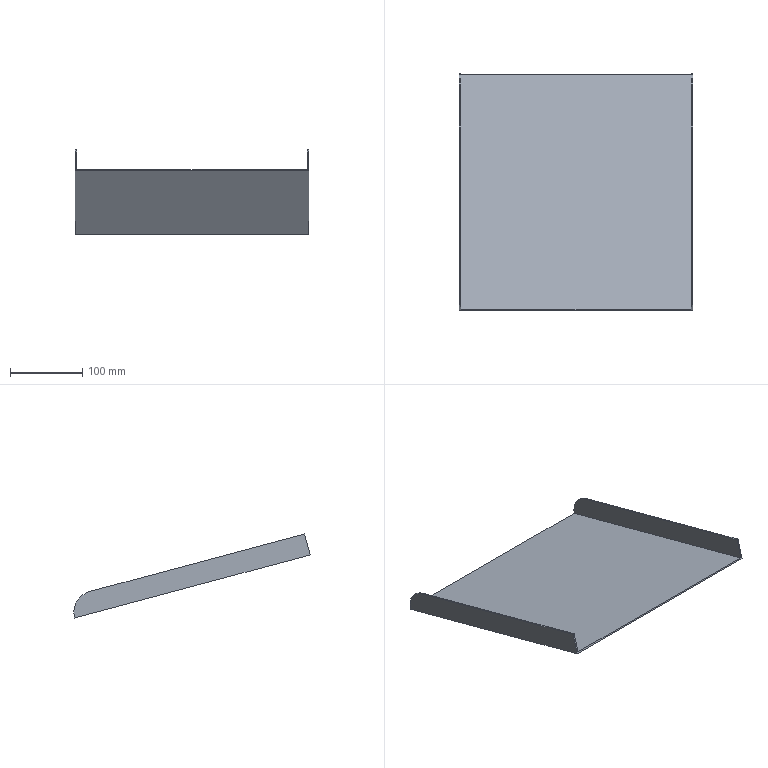Part | NX | features solid 2 | 1 solid | 12 faces | box 322.884 x 327.249 x 116.39 mm | volume 255152 mm3 | plane 9 | cylinder 2 | spline 1 | commonest cylinder face diameters 60 x2
STEP:
#1=CARTESIAN_POINT('',(-1268.,804.132,-484.555));
#2=VERTEX_POINT('',#1);
#3=CARTESIAN_POINT('',(-1268.,1130.294,-571.95));
#4=VERTEX_POINT('',#3);
#5=CARTESIAN_POINT('',(-1268.,966.151,-527.968));
#6=DIRECTION('',(0.,0.9659,-0.2588));
#7=VECTOR('',#6,1000.);
#8=LINE('',#5,#7);
#9=EDGE_CURVE('',#2,#4,#8,.T.);
#10=ORIENTED_EDGE('',*,*,#9,.F.);
#11=CARTESIAN_POINT('',(-949.116,804.132,-484.555));
#12=VERTEX_POINT('',#11);
#13=CARTESIAN_POINT('',(-1258.,804.132,-484.555));
#14=DIRECTION('',(1.,0.,0.));
#15=VECTOR('',#14,1000.);
#16=LINE('',#13,#15);
#17=EDGE_CURVE('',#2,#12,#16,.T.);
#18=ORIENTED_EDGE('',*,*,#17,.T.);
#19=CARTESIAN_POINT('',(-949.116,1130.294,-571.95));
#20=VERTEX_POINT('',#19);
#21=CARTESIAN_POINT('',(-949.116,966.151,-527.968));
#22=DIRECTION('',(0.,0.9659,-0.2588));
#23=VECTOR('',#22,1000.);
#24=LINE('',#21,#23);
#25=EDGE_CURVE('',#12,#20,#24,.T.);
#26=ORIENTED_EDGE('',*,*,#25,.T.);
#27=CARTESIAN_POINT('',(-947.116,1130.294,-571.95));
#28=VERTEX_POINT('',#27);
#29=CARTESIAN_POINT('',(-947.116,1130.294,-571.95));
#30=DIRECTION('',(1.,0.,0.));
#31=VECTOR('',#30,1000.);
#32=LINE('',#29,#31);
#33=EDGE_CURVE('',#28,#20,#32,.F.);
#34=ORIENTED_EDGE('',*,*,#33,.F.);
#35=CARTESIAN_POINT('',(-947.116,1130.359,-571.967));
#36=VERTEX_POINT('',#35);
#37=CARTESIAN_POINT('',(-947.116,966.151,-527.968));
#38=DIRECTION('',(0.,-0.9659,0.2588));
#39=VECTOR('',#38,1000.);
#40=LINE('',#37,#39);
#41=EDGE_CURVE('',#28,#36,#40,.F.);
#42=ORIENTED_EDGE('',*,*,#41,.T.);
#43=CARTESIAN_POINT('',(-1270.,1130.359,-571.967));
#44=VERTEX_POINT('',#43);
#45=CARTESIAN_POINT('',(-1302.833,1130.359,-571.967));
#46=CARTESIAN_POINT('',(-1258.,1130.359,-571.967));
#47=CARTESIAN_POINT('',(-959.116,1130.359,-571.967));
#48=CARTESIAN_POINT('',(-914.283,1130.359,-571.967));
#49=B_SPLINE_CURVE_WITH_KNOTS('',1,(#45,#46,#47,#48),.UNSPECIFIED.,.F.,.F.,(2,1,1,2),(-0.15,0.,1.,1.15),.PIECEWISE_BEZIER_KNOTS.);
#50=EDGE_CURVE('',#44,#36,#49,.T.);
#51=ORIENTED_EDGE('',*,*,#50,.F.);
#52=CARTESIAN_POINT('',(-1270.,1130.294,-571.95));
#53=VERTEX_POINT('',#52);
#54=CARTESIAN_POINT('',(-1270.,966.151,-527.968));
#55=DIRECTION('',(0.,0.9659,-0.2588));
#56=VECTOR('',#55,1000.);
#57=LINE('',#54,#56);
#58=EDGE_CURVE('',#53,#44,#57,.T.);
#59=ORIENTED_EDGE('',*,*,#58,.F.);
#60=CARTESIAN_POINT('',(-1270.,1130.294,-571.95));
#61=DIRECTION('',(-1.,0.,0.));
#62=VECTOR('',#61,1000.);
#63=LINE('',#60,#62);
#64=EDGE_CURVE('',#4,#53,#63,.T.);
#65=ORIENTED_EDGE('',*,*,#64,.F.);
#66=EDGE_LOOP('',(#10,#18,#26,#34,#42,#51,#59,#65));
#67=FACE_BOUND('',#66,.T.);
#68=CARTESIAN_POINT('',(-1258.,966.151,-527.968));
#69=DIRECTION('',(0.,0.2588,0.9659));
#70=DIRECTION('',(1.,0.,0.));
#71=AXIS2_PLACEMENT_3D('',#68,#69,#70);
#72=PLANE('',#71);
#73=ADVANCED_FACE('',(#67),#72,.T.);
#74=CARTESIAN_POINT('',(-947.116,803.615,-486.487));
#75=VERTEX_POINT('',#74);
#76=CARTESIAN_POINT('',(-947.116,811.379,-457.509));
#77=VERTEX_POINT('',#76);
#78=CARTESIAN_POINT('',(-947.116,804.132,-484.555));
#79=DIRECTION('',(0.,-0.2588,-0.9659));
#80=VECTOR('',#79,1000.);
#81=LINE('',#78,#80);
#82=EDGE_CURVE('',#75,#77,#81,.F.);
#83=ORIENTED_EDGE('',*,*,#82,.F.);
#84=CARTESIAN_POINT('',(-947.116,1129.841,-573.899));
#85=VERTEX_POINT('',#84);
#86=CARTESIAN_POINT('',(-947.116,965.634,-529.9));
#87=DIRECTION('',(0.,-0.9659,0.2588));
#88=VECTOR('',#87,1000.);
#89=LINE('',#86,#88);
#90=EDGE_CURVE('',#75,#85,#89,.F.);
#91=ORIENTED_EDGE('',*,*,#90,.T.);
#92=CARTESIAN_POINT('',(-947.116,1130.1,-572.933));
#93=DIRECTION('',(0.,0.2588,0.9659));
#94=VECTOR('',#93,1000.);
#95=LINE('',#92,#94);
#96=EDGE_CURVE('',#36,#85,#95,.F.);
#97=ORIENTED_EDGE('',*,*,#96,.F.);
#98=ORIENTED_EDGE('',*,*,#41,.F.);
#99=CARTESIAN_POINT('',(-947.116,1108.628,-537.157));
#100=VERTEX_POINT('',#99);
#101=CARTESIAN_POINT('',(-947.116,1100.863,-566.134));
#102=DIRECTION('',(1.,0.,0.));
#103=DIRECTION('',(0.,0.08716,-0.9962));
#104=AXIS2_PLACEMENT_3D('',#101,#102,#103);
#105=CIRCLE('',#104,30.);
#106=EDGE_CURVE('',#28,#100,#105,.T.);
#107=ORIENTED_EDGE('',*,*,#106,.T.);
#108=CARTESIAN_POINT('',(-947.116,944.421,-493.157));
#109=DIRECTION('',(0.,0.9659,-0.2588));
#110=VECTOR('',#109,1000.);
#111=LINE('',#108,#110);
#112=EDGE_CURVE('',#77,#100,#111,.T.);
#113=ORIENTED_EDGE('',*,*,#112,.F.);
#114=EDGE_LOOP('',(#83,#91,#97,#98,#107,#113));
#115=FACE_BOUND('',#114,.T.);
#116=CARTESIAN_POINT('',(-947.116,966.151,-527.968));
#117=DIRECTION('',(1.,0.,0.));
#118=DIRECTION('',(0.,0.9659,-0.2588));
#119=AXIS2_PLACEMENT_3D('',#116,#117,#118);
#120=PLANE('',#119);
#121=ADVANCED_FACE('',(#115),#120,.T.);
#122=CARTESIAN_POINT('',(-1270.,811.379,-457.509));
#123=VERTEX_POINT('',#122);
#124=CARTESIAN_POINT('',(-1270.,803.615,-486.487));
#125=VERTEX_POINT('',#124);
#126=CARTESIAN_POINT('',(-1270.,804.132,-484.555));
#127=DIRECTION('',(0.,-0.2588,-0.9659));
#128=VECTOR('',#127,1000.);
#129=LINE('',#126,#128);
#130=EDGE_CURVE('',#123,#125,#129,.T.);
#131=ORIENTED_EDGE('',*,*,#130,.F.);
#132=CARTESIAN_POINT('',(-1270.,1108.628,-537.157));
#133=VERTEX_POINT('',#132);
#134=CARTESIAN_POINT('',(-1270.,944.421,-493.157));
#135=DIRECTION('',(0.,0.9659,-0.2588));
#136=VECTOR('',#135,1000.);
#137=LINE('',#134,#136);
#138=EDGE_CURVE('',#123,#133,#137,.T.);
#139=ORIENTED_EDGE('',*,*,#138,.T.);
#140=CARTESIAN_POINT('',(-1270.,1100.863,-566.134));
#141=DIRECTION('',(1.,0.,0.));
#142=DIRECTION('',(0.,0.08716,-0.9962));
#143=AXIS2_PLACEMENT_3D('',#140,#141,#142);
#144=CIRCLE('',#143,30.);
#145=EDGE_CURVE('',#133,#53,#144,.F.);
#146=ORIENTED_EDGE('',*,*,#145,.T.);
#147=ORIENTED_EDGE('',*,*,#58,.T.);
#148=CARTESIAN_POINT('',(-1270.,1129.841,-573.899));
#149=VERTEX_POINT('',#148);
#150=CARTESIAN_POINT('',(-1270.,1130.359,-571.967));
#151=DIRECTION('',(0.,0.2588,0.9659));
#152=VECTOR('',#151,1000.);
#153=LINE('',#150,#152);
#154=EDGE_CURVE('',#44,#149,#153,.F.);
#155=ORIENTED_EDGE('',*,*,#154,.T.);
#156=CARTESIAN_POINT('',(-1270.,965.634,-529.9));
#157=DIRECTION('',(0.,0.9659,-0.2588));
#158=VECTOR('',#157,1000.);
#159=LINE('',#156,#158);
#160=EDGE_CURVE('',#125,#149,#159,.T.);
#161=ORIENTED_EDGE('',*,*,#160,.F.);
#162=EDGE_LOOP('',(#131,#139,#146,#147,#155,#161));
#163=FACE_BOUND('',#162,.T.);
#164=CARTESIAN_POINT('',(-1270.,966.151,-527.968));
#165=DIRECTION('',(1.,0.,0.));
#166=DIRECTION('',(0.,0.9659,-0.2588));
#167=AXIS2_PLACEMENT_3D('',#164,#165,#166);
#168=PLANE('',#167);
#169=ADVANCED_FACE('',(#163),#168,.F.);
#170=CARTESIAN_POINT('',(-1258.,803.615,-486.487));
#171=DIRECTION('',(1.,0.,0.));
#172=VECTOR('',#171,1000.);
#173=LINE('',#170,#172);
#174=EDGE_CURVE('',#125,#75,#173,.T.);
#175=ORIENTED_EDGE('',*,*,#174,.F.);
#176=ORIENTED_EDGE('',*,*,#160,.T.);
#177=CARTESIAN_POINT('',(-1302.833,1129.841,-573.899));
#178=CARTESIAN_POINT('',(-1258.,1129.841,-573.899));
#179=CARTESIAN_POINT('',(-959.116,1129.841,-573.899));
#180=CARTESIAN_POINT('',(-914.283,1129.841,-573.899));
#181=B_SPLINE_CURVE_WITH_KNOTS('',1,(#177,#178,#179,#180),.UNSPECIFIED.,.F.,.F.,(2,1,1,2),(-0.15,0.,1.,1.15),.PIECEWISE_BEZIER_KNOTS.);
#182=EDGE_CURVE('',#149,#85,#181,.T.);
#183=ORIENTED_EDGE('',*,*,#182,.T.);
#184=ORIENTED_EDGE('',*,*,#90,.F.);
#185=EDGE_LOOP('',(#175,#176,#183,#184));
#186=FACE_BOUND('',#185,.T.);
#187=CARTESIAN_POINT('',(-1258.,965.634,-529.9));
#188=DIRECTION('',(0.,0.2588,0.9659));
#189=DIRECTION('',(1.,0.,0.));
#190=AXIS2_PLACEMENT_3D('',#187,#188,#189);
#191=PLANE('',#190);
#192=ADVANCED_FACE('',(#186),#191,.F.);
#193=CARTESIAN_POINT('',(-949.116,811.379,-457.509));
#194=VERTEX_POINT('',#193);
#195=CARTESIAN_POINT('',(-947.116,811.379,-457.509));
#196=DIRECTION('',(-1.,0.,0.));
#197=VECTOR('',#196,1000.);
#198=LINE('',#195,#197);
#199=EDGE_CURVE('',#77,#194,#198,.T.);
#200=ORIENTED_EDGE('',*,*,#199,.F.);
#201=ORIENTED_EDGE('',*,*,#112,.T.);
#202=CARTESIAN_POINT('',(-949.116,1108.628,-537.157));
#203=VERTEX_POINT('',#202);
#204=CARTESIAN_POINT('',(-947.116,1108.628,-537.157));
#205=DIRECTION('',(1.,0.,0.));
#206=VECTOR('',#205,1000.);
#207=LINE('',#204,#206);
#208=EDGE_CURVE('',#100,#203,#207,.F.);
#209=ORIENTED_EDGE('',*,*,#208,.T.);
#210=CARTESIAN_POINT('',(-949.116,944.421,-493.157));
#211=DIRECTION('',(0.,0.9659,-0.2588));
#212=VECTOR('',#211,1000.);
#213=LINE('',#210,#212);
#214=EDGE_CURVE('',#194,#203,#213,.T.);
#215=ORIENTED_EDGE('',*,*,#214,.F.);
#216=EDGE_LOOP('',(#200,#201,#209,#215));
#217=FACE_BOUND('',#216,.T.);
#218=CARTESIAN_POINT('',(-947.116,944.421,-493.157));
#219=DIRECTION('',(0.,-0.2588,-0.9659));
#220=DIRECTION('',(0.,0.9659,-0.2588));
#221=AXIS2_PLACEMENT_3D('',#218,#219,#220);
#222=PLANE('',#221);
#223=ADVANCED_FACE('',(#217),#222,.F.);
#224=CARTESIAN_POINT('',(-949.116,803.615,-486.487));
#225=DIRECTION('',(0.,-0.2588,-0.9659));
#226=VECTOR('',#225,1000.);
#227=LINE('',#224,#226);
#228=EDGE_CURVE('',#194,#12,#227,.T.);
#229=ORIENTED_EDGE('',*,*,#228,.F.);
#230=ORIENTED_EDGE('',*,*,#214,.T.);
#231=CARTESIAN_POINT('',(-949.116,1100.863,-566.134));
#232=DIRECTION('',(1.,0.,0.));
#233=DIRECTION('',(0.,0.08716,-0.9962));
#234=AXIS2_PLACEMENT_3D('',#231,#232,#233);
#235=CIRCLE('',#234,30.);
#236=EDGE_CURVE('',#203,#20,#235,.F.);
#237=ORIENTED_EDGE('',*,*,#236,.T.);
#238=ORIENTED_EDGE('',*,*,#25,.F.);
#239=EDGE_LOOP('',(#229,#230,#237,#238));
#240=FACE_BOUND('',#239,.T.);
#241=CARTESIAN_POINT('',(-949.116,936.656,-522.135));
#242=DIRECTION('',(1.,0.,0.));
#243=DIRECTION('',(0.,0.08716,-0.9962));
#244=AXIS2_PLACEMENT_3D('',#241,#242,#243);
#245=PLANE('',#244);
#246=ADVANCED_FACE('',(#240),#245,.F.);
#247=ORIENTED_EDGE('',*,*,#138,.F.);
#248=CARTESIAN_POINT('',(-1268.,811.379,-457.509));
#249=VERTEX_POINT('',#248);
#250=CARTESIAN_POINT('',(-1270.,811.379,-457.509));
#251=DIRECTION('',(-1.,0.,0.));
#252=VECTOR('',#251,1000.);
#253=LINE('',#250,#252);
#254=EDGE_CURVE('',#123,#249,#253,.F.);
#255=ORIENTED_EDGE('',*,*,#254,.T.);
#256=CARTESIAN_POINT('',(-1268.,1108.628,-537.157));
#257=VERTEX_POINT('',#256);
#258=CARTESIAN_POINT('',(-1268.,944.421,-493.157));
#259=DIRECTION('',(0.,0.9659,-0.2588));
#260=VECTOR('',#259,1000.);
#261=LINE('',#258,#260);
#262=EDGE_CURVE('',#249,#257,#261,.T.);
#263=ORIENTED_EDGE('',*,*,#262,.T.);
#264=CARTESIAN_POINT('',(-1270.,1108.628,-537.157));
#265=DIRECTION('',(1.,0.,0.));
#266=VECTOR('',#265,1000.);
#267=LINE('',#264,#266);
#268=EDGE_CURVE('',#257,#133,#267,.F.);
#269=ORIENTED_EDGE('',*,*,#268,.T.);
#270=EDGE_LOOP('',(#247,#255,#263,#269));
#271=FACE_BOUND('',#270,.T.);
#272=CARTESIAN_POINT('',(-1270.,944.421,-493.157));
#273=DIRECTION('',(0.,-0.2588,-0.9659));
#274=DIRECTION('',(0.,0.9659,-0.2588));
#275=AXIS2_PLACEMENT_3D('',#272,#273,#274);
#276=PLANE('',#275);
#277=ADVANCED_FACE('',(#271),#276,.F.);
#278=ORIENTED_EDGE('',*,*,#262,.F.);
#279=CARTESIAN_POINT('',(-1268.,803.615,-486.487));
#280=DIRECTION('',(0.,-0.2588,-0.9659));
#281=VECTOR('',#280,1000.);
#282=LINE('',#279,#281);
#283=EDGE_CURVE('',#249,#2,#282,.T.);
#284=ORIENTED_EDGE('',*,*,#283,.T.);
#285=ORIENTED_EDGE('',*,*,#9,.T.);
#286=CARTESIAN_POINT('',(-1268.,1100.863,-566.134));
#287=DIRECTION('',(1.,0.,0.));
#288=DIRECTION('',(0.,0.08716,-0.9962));
#289=AXIS2_PLACEMENT_3D('',#286,#287,#288);
#290=CIRCLE('',#289,30.);
#291=EDGE_CURVE('',#4,#257,#290,.T.);
#292=ORIENTED_EDGE('',*,*,#291,.T.);
#293=EDGE_LOOP('',(#278,#284,#285,#292));
#294=FACE_BOUND('',#293,.T.);
#295=CARTESIAN_POINT('',(-1268.,936.656,-522.135));
#296=DIRECTION('',(1.,0.,0.));
#297=DIRECTION('',(0.,0.08716,-0.9962));
#298=AXIS2_PLACEMENT_3D('',#295,#296,#297);
#299=PLANE('',#298);
#300=ADVANCED_FACE('',(#294),#299,.T.);
#301=ORIENTED_EDGE('',*,*,#96,.T.);
#302=ORIENTED_EDGE('',*,*,#182,.F.);
#303=ORIENTED_EDGE('',*,*,#154,.F.);
#304=ORIENTED_EDGE('',*,*,#50,.T.);
#305=EDGE_LOOP('',(#301,#302,#303,#304));
#306=FACE_BOUND('',#305,.T.);
#307=CARTESIAN_POINT('',(-1270.,1129.841,-573.899));
#308=CARTESIAN_POINT('',(-1270.,1130.359,-571.967));
#309=CARTESIAN_POINT('',(-1258.,1129.841,-573.899));
#310=CARTESIAN_POINT('',(-1258.,1130.359,-571.967));
#311=CARTESIAN_POINT('',(-959.116,1129.841,-573.899));
#312=CARTESIAN_POINT('',(-959.116,1130.359,-571.967));
#313=CARTESIAN_POINT('',(-947.116,1129.841,-573.899));
#314=CARTESIAN_POINT('',(-947.116,1130.359,-571.967));
#315=B_SPLINE_SURFACE_WITH_KNOTS('',1,1,((#307,#308),(#309,#310),(#311,#312),(#313,#314)),.SURF_OF_LINEAR_EXTRUSION.,.F.,.F.,.F.,(2,1,1,2),(2,2),(-0.04015,0.,1.,1.04),(0.,1.),.PIECEWISE_BEZIER_KNOTS.);
#316=ADVANCED_FACE('',(#306),#315,.F.);
#317=ORIENTED_EDGE('',*,*,#106,.F.);
#318=ORIENTED_EDGE('',*,*,#33,.T.);
#319=ORIENTED_EDGE('',*,*,#236,.F.);
#320=ORIENTED_EDGE('',*,*,#208,.F.);
#321=EDGE_LOOP('',(#317,#318,#319,#320));
#322=FACE_BOUND('',#321,.T.);
#323=CARTESIAN_POINT('',(-947.116,1100.863,-566.134));
#324=DIRECTION('',(1.,0.,0.));
#325=DIRECTION('',(0.,0.08716,-0.9962));
#326=AXIS2_PLACEMENT_3D('',#323,#324,#325);
#327=CYLINDRICAL_SURFACE('',#326,30.);
#328=ADVANCED_FACE('',(#322),#327,.T.);
#329=ORIENTED_EDGE('',*,*,#291,.F.);
#330=ORIENTED_EDGE('',*,*,#64,.T.);
#331=ORIENTED_EDGE('',*,*,#145,.F.);
#332=ORIENTED_EDGE('',*,*,#268,.F.);
#333=EDGE_LOOP('',(#329,#330,#331,#332));
#334=FACE_BOUND('',#333,.T.);
#335=CARTESIAN_POINT('',(-1270.,1100.863,-566.134));
#336=DIRECTION('',(-1.,0.,0.));
#337=DIRECTION('',(0.,-0.08716,0.9962));
#338=AXIS2_PLACEMENT_3D('',#335,#336,#337);
#339=CYLINDRICAL_SURFACE('',#338,30.);
#340=ADVANCED_FACE('',(#334),#339,.T.);
#341=ORIENTED_EDGE('',*,*,#174,.T.);
#342=ORIENTED_EDGE('',*,*,#82,.T.);
#343=ORIENTED_EDGE('',*,*,#199,.T.);
#344=ORIENTED_EDGE('',*,*,#228,.T.);
#345=ORIENTED_EDGE('',*,*,#17,.F.);
#346=ORIENTED_EDGE('',*,*,#283,.F.);
#347=ORIENTED_EDGE('',*,*,#254,.F.);
#348=ORIENTED_EDGE('',*,*,#130,.T.);
#349=EDGE_LOOP('',(#341,#342,#343,#344,#345,#346,#347,#348));
#350=FACE_BOUND('',#349,.T.);
#351=CARTESIAN_POINT('',(-1270.,811.379,-457.509));
#352=DIRECTION('',(0.,-0.9659,0.2588));
#353=DIRECTION('',(0.,-0.2588,-0.9659));
#354=AXIS2_PLACEMENT_3D('',#351,#352,#353);
#355=PLANE('',#354);
#356=ADVANCED_FACE('',(#350),#355,.T.);
#357=CLOSED_SHELL('',(#73,#121,#169,#192,#223,#246,#277,#300,#316,#328,#340,#356));
#358=MANIFOLD_SOLID_BREP('',#357);
#359=(LENGTH_UNIT()NAMED_UNIT(*)SI_UNIT(.MILLI.,.METRE.));
#360=UNCERTAINTY_MEASURE_WITH_UNIT(LENGTH_MEASURE(0.0508),#359,'','');
#361=(NAMED_UNIT(*)PLANE_ANGLE_UNIT()SI_UNIT($,.RADIAN.));
#362=(NAMED_UNIT(*)SI_UNIT($,.STERADIAN.)SOLID_ANGLE_UNIT());
#363=(GEOMETRIC_REPRESENTATION_CONTEXT(3)GLOBAL_UNCERTAINTY_ASSIGNED_CONTEXT((#360))GLOBAL_UNIT_ASSIGNED_CONTEXT((#359,#361,#362))REPRESENTATION_CONTEXT('',''));
#364=ADVANCED_BREP_SHAPE_REPRESENTATION('',(#358),#363);